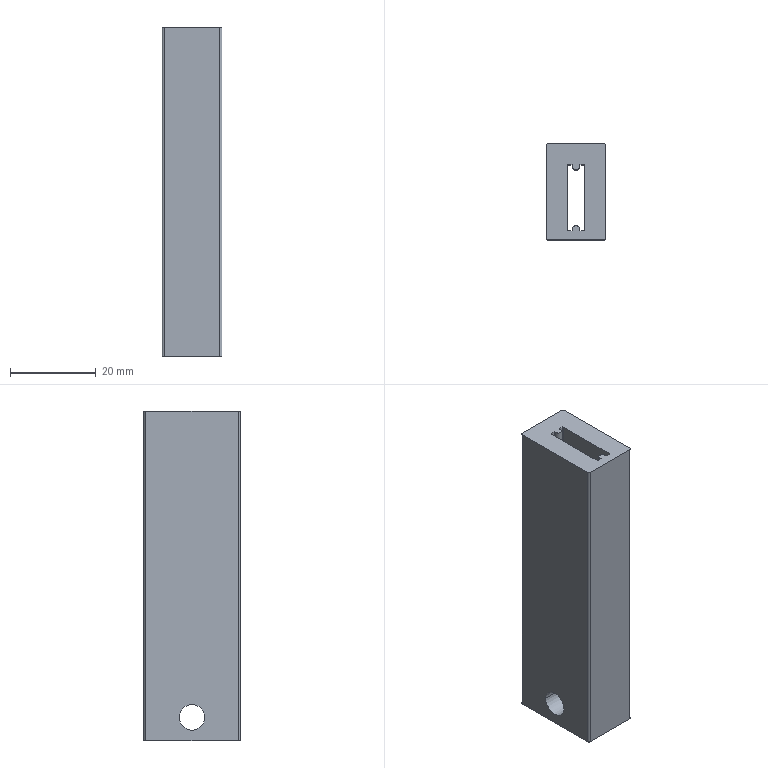Part | STEP file | THAN GA LUOI DOT | 1 solid | 36 faces | box 14 x 22.5 x 77 mm | volume 19378 mm3 | cylinder 20 | plane 16 | commonest cylinder face diameters 0.2 x4 0.4 x4 1 x4 6 x4 1.6 x2 4.3 x2